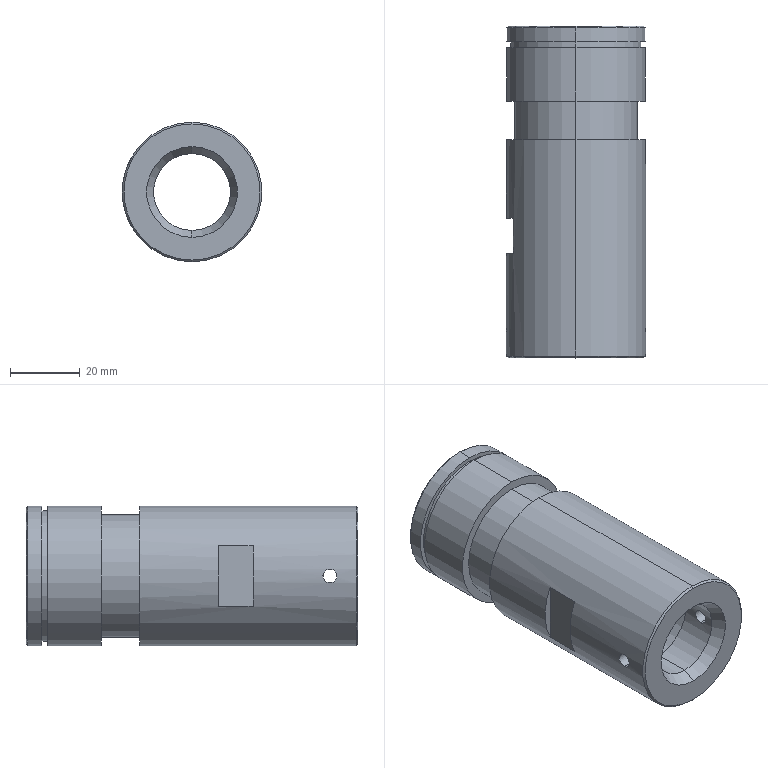Part | SolidWorks | features Chamfer 2, ICE 2, 3DProfileFeature 1, Extrusion 1, HoleWzd 1, RevCut 1 | 1 solid | 36 faces | box 40 x 95 x 40 mm | volume 59618 mm3 | cylinder 18 | plane 10 | cone 8 | commonest cylinder face diameters 40 x6 4 x4 22 x2 28 x2 35 x2 37.5 x2
STEP:
#1=CARTESIAN_POINT('',(0.,91.536,-14.));
#2=VERTEX_POINT('',#1);
#3=CARTESIAN_POINT('',(0.,91.536,14.));
#4=VERTEX_POINT('',#3);
#5=CARTESIAN_POINT('',(0.,91.536,0.));
#6=DIRECTION('',(0.,1.,0.));
#7=DIRECTION('',(0.,0.,1.));
#8=AXIS2_PLACEMENT_3D('',#5,#6,#7);
#9=CIRCLE('',#8,14.);
#10=EDGE_CURVE('',#2,#4,#9,.T.);
#11=ORIENTED_EDGE('',*,*,#10,.F.);
#12=CARTESIAN_POINT('',(0.,95.,-16.));
#13=VERTEX_POINT('',#12);
#14=CARTESIAN_POINT('',(0.,91.536,-14.));
#15=DIRECTION('',(0.,0.866,-0.5));
#16=VECTOR('',#15,1000.);
#17=LINE('',#14,#16);
#18=EDGE_CURVE('',#2,#13,#17,.T.);
#19=ORIENTED_EDGE('',*,*,#18,.T.);
#20=CARTESIAN_POINT('',(0.,95.,16.));
#21=VERTEX_POINT('',#20);
#22=CARTESIAN_POINT('',(0.,95.,0.));
#23=DIRECTION('',(0.,-1.,0.));
#24=DIRECTION('',(0.,0.,1.));
#25=AXIS2_PLACEMENT_3D('',#22,#23,#24);
#26=CIRCLE('',#25,16.);
#27=EDGE_CURVE('',#21,#13,#26,.T.);
#28=ORIENTED_EDGE('',*,*,#27,.F.);
#29=CARTESIAN_POINT('',(0.,91.536,14.));
#30=DIRECTION('',(0.,0.866,0.5));
#31=VECTOR('',#30,1000.);
#32=LINE('',#29,#31);
#33=EDGE_CURVE('',#4,#21,#32,.T.);
#34=ORIENTED_EDGE('',*,*,#33,.F.);
#35=EDGE_LOOP('',(#11,#19,#28,#34));
#36=FACE_OUTER_BOUND('',#35,.T.);
#37=CARTESIAN_POINT('',(0.,91.536,0.));
#38=DIRECTION('',(0.,1.,0.));
#39=DIRECTION('',(0.,0.,1.));
#40=AXIS2_PLACEMENT_3D('',#37,#38,#39);
#41=CONICAL_SURFACE('',#40,14.,0.5236);
#42=ADVANCED_FACE('',(#36),#41,.F.);
#43=CARTESIAN_POINT('',(0.,3.464,11.));
#44=VERTEX_POINT('',#43);
#45=CARTESIAN_POINT('',(0.,3.464,-11.));
#46=VERTEX_POINT('',#45);
#47=CARTESIAN_POINT('',(0.,3.464,0.));
#48=DIRECTION('',(0.,-1.,0.));
#49=DIRECTION('',(0.,0.,1.));
#50=AXIS2_PLACEMENT_3D('',#47,#48,#49);
#51=CIRCLE('',#50,11.);
#52=EDGE_CURVE('',#44,#46,#51,.T.);
#53=ORIENTED_EDGE('',*,*,#52,.F.);
#54=CARTESIAN_POINT('',(0.,0.,13.));
#55=VERTEX_POINT('',#54);
#56=CARTESIAN_POINT('',(0.,3.464,11.));
#57=DIRECTION('',(0.,-0.866,0.5));
#58=VECTOR('',#57,1000.);
#59=LINE('',#56,#58);
#60=EDGE_CURVE('',#44,#55,#59,.T.);
#61=ORIENTED_EDGE('',*,*,#60,.T.);
#62=CARTESIAN_POINT('',(0.,0.,-13.));
#63=VERTEX_POINT('',#62);
#64=CARTESIAN_POINT('',(0.,0.,0.));
#65=DIRECTION('',(0.,1.,0.));
#66=DIRECTION('',(0.,0.,1.));
#67=AXIS2_PLACEMENT_3D('',#64,#65,#66);
#68=CIRCLE('',#67,13.);
#69=EDGE_CURVE('',#63,#55,#68,.T.);
#70=ORIENTED_EDGE('',*,*,#69,.F.);
#71=CARTESIAN_POINT('',(0.,3.464,-11.));
#72=DIRECTION('',(0.,-0.866,-0.5));
#73=VECTOR('',#72,1000.);
#74=LINE('',#71,#73);
#75=EDGE_CURVE('',#46,#63,#74,.T.);
#76=ORIENTED_EDGE('',*,*,#75,.F.);
#77=EDGE_LOOP('',(#53,#61,#70,#76));
#78=FACE_OUTER_BOUND('',#77,.T.);
#79=CARTESIAN_POINT('',(0.,3.464,0.));
#80=DIRECTION('',(0.,-1.,0.));
#81=DIRECTION('',(0.,0.,-1.));
#82=AXIS2_PLACEMENT_3D('',#79,#80,#81);
#83=CONICAL_SURFACE('',#82,11.,0.5236);
#84=ADVANCED_FACE('',(#78),#83,.F.);
#85=CARTESIAN_POINT('',(-19.9,8.,2.));
#86=VERTEX_POINT('',#85);
#87=CARTESIAN_POINT('',(-19.9,8.,-2.));
#88=VERTEX_POINT('',#87);
#89=CARTESIAN_POINT('',(-19.9,8.,2.));
#90=CARTESIAN_POINT('',(-19.9,7.868,2.));
#91=CARTESIAN_POINT('',(-19.901,7.738,1.987));
#92=CARTESIAN_POINT('',(-19.906,7.482,1.936));
#93=CARTESIAN_POINT('',(-19.91,7.355,1.898));
#94=CARTESIAN_POINT('',(-19.919,7.113,1.797));
#95=CARTESIAN_POINT('',(-19.925,6.998,1.736));
#96=CARTESIAN_POINT('',(-19.937,6.781,1.591));
#97=CARTESIAN_POINT('',(-19.943,6.678,1.506));
#98=CARTESIAN_POINT('',(-19.963,6.401,1.23));
#99=CARTESIAN_POINT('',(-19.976,6.252,1.007));
#100=CARTESIAN_POINT('',(-19.995,6.053,0.5256));
#101=CARTESIAN_POINT('',(-20.,6.,0.2629));
#102=CARTESIAN_POINT('',(-20.,6.,-0.1337));
#103=CARTESIAN_POINT('',(-19.999,6.013,-0.2637));
#104=CARTESIAN_POINT('',(-19.994,6.064,-0.5193));
#105=CARTESIAN_POINT('',(-19.99,6.103,-0.6463));
#106=CARTESIAN_POINT('',(-19.981,6.203,-0.8884));
#107=CARTESIAN_POINT('',(-19.975,6.265,-1.003));
#108=CARTESIAN_POINT('',(-19.963,6.41,-1.22));
#109=CARTESIAN_POINT('',(-19.956,6.495,-1.323));
#110=CARTESIAN_POINT('',(-19.937,6.771,-1.599));
#111=CARTESIAN_POINT('',(-19.924,6.994,-1.748));
#112=CARTESIAN_POINT('',(-19.905,7.476,-1.948));
#113=CARTESIAN_POINT('',(-19.9,7.739,-2.));
#114=CARTESIAN_POINT('',(-19.9,8.,-2.));
#115=B_SPLINE_CURVE_WITH_KNOTS('',3,(#89,#90,#91,#92,#93,#94,#95,#96,#97,#98,#99,#100,#101,#102,#103,#104,#105,#106,#107,#108,#109,#110,#111,#112,#113,#114),.UNSPECIFIED.,.F.,.F.,(4,2,2,2,2,2,2,2,2,2,2,2,4),(0.009386,0.009777,0.01017,0.01056,0.01095,0.01173,0.01251,0.0129,0.0133,0.01369,0.01408,0.01486,0.01564),.UNSPECIFIED.);
#116=EDGE_CURVE('',#86,#88,#115,.T.);
#117=ORIENTED_EDGE('',*,*,#116,.F.);
#118=CARTESIAN_POINT('',(-10.817,8.,2.));
#119=VERTEX_POINT('',#118);
#120=CARTESIAN_POINT('',(20.,8.,2.));
#121=DIRECTION('',(1.,0.,0.));
#122=VECTOR('',#121,1000.);
#123=LINE('',#120,#122);
#124=EDGE_CURVE('',#86,#119,#123,.T.);
#125=ORIENTED_EDGE('',*,*,#124,.T.);
#126=CARTESIAN_POINT('',(-10.817,8.,-2.));
#127=VERTEX_POINT('',#126);
#128=CARTESIAN_POINT('',(-10.817,8.,-2.));
#129=CARTESIAN_POINT('',(-10.817,7.868,-2.));
#130=CARTESIAN_POINT('',(-10.819,7.737,-1.987));
#131=CARTESIAN_POINT('',(-10.828,7.481,-1.936));
#132=CARTESIAN_POINT('',(-10.835,7.354,-1.897));
#133=CARTESIAN_POINT('',(-10.852,7.112,-1.797));
#134=CARTESIAN_POINT('',(-10.862,6.997,-1.735));
#135=CARTESIAN_POINT('',(-10.885,6.78,-1.59));
#136=CARTESIAN_POINT('',(-10.897,6.678,-1.506));
#137=CARTESIAN_POINT('',(-10.933,6.401,-1.23));
#138=CARTESIAN_POINT('',(-10.956,6.253,-1.007));
#139=CARTESIAN_POINT('',(-10.99,6.053,-0.5259));
#140=CARTESIAN_POINT('',(-11.,6.,-0.2623));
#141=CARTESIAN_POINT('',(-11.,6.,0.13));
#142=CARTESIAN_POINT('',(-10.998,6.013,0.2628));
#143=CARTESIAN_POINT('',(-10.988,6.064,0.5196));
#144=CARTESIAN_POINT('',(-10.982,6.102,0.6444));
#145=CARTESIAN_POINT('',(-10.965,6.203,0.8869));
#146=CARTESIAN_POINT('',(-10.955,6.265,1.004));
#147=CARTESIAN_POINT('',(-10.933,6.41,1.22));
#148=CARTESIAN_POINT('',(-10.921,6.493,1.321));
#149=CARTESIAN_POINT('',(-10.897,6.679,1.507));
#150=CARTESIAN_POINT('',(-10.885,6.78,1.59));
#151=CARTESIAN_POINT('',(-10.863,6.996,1.735));
#152=CARTESIAN_POINT('',(-10.852,7.113,1.797));
#153=CARTESIAN_POINT('',(-10.835,7.355,1.898));
#154=CARTESIAN_POINT('',(-10.828,7.48,1.936));
#155=CARTESIAN_POINT('',(-10.819,7.737,1.987));
#156=CARTESIAN_POINT('',(-10.817,7.869,2.));
#157=CARTESIAN_POINT('',(-10.817,8.,2.));
#158=B_SPLINE_CURVE_WITH_KNOTS('',3,(#128,#129,#130,#131,#132,#133,#134,#135,#136,#137,#138,#139,#140,#141,#142,#143,#144,#145,#146,#147,#148,#149,#150,#151,#152,#153,#154,#155,#156,#157),.UNSPECIFIED.,.F.,.F.,(4,2,2,2,2,2,2,2,2,2,2,2,2,2,4),(0.,0.0003916,0.0007832,0.001175,0.001566,0.00235,0.003133,0.003525,0.003916,0.004308,0.004699,0.005091,0.005483,0.005874,0.006266),.UNSPECIFIED.);
#159=EDGE_CURVE('',#127,#119,#158,.T.);
#160=ORIENTED_EDGE('',*,*,#159,.F.);
#161=CARTESIAN_POINT('',(20.,8.,-2.));
#162=DIRECTION('',(1.,0.,0.));
#163=VECTOR('',#162,1000.);
#164=LINE('',#161,#163);
#165=EDGE_CURVE('',#88,#127,#164,.T.);
#166=ORIENTED_EDGE('',*,*,#165,.F.);
#167=EDGE_LOOP('',(#117,#125,#160,#166));
#168=FACE_OUTER_BOUND('',#167,.T.);
#169=CARTESIAN_POINT('',(20.,8.,0.));
#170=DIRECTION('',(1.,0.,0.));
#171=DIRECTION('',(0.,0.,-1.));
#172=AXIS2_PLACEMENT_3D('',#169,#170,#171);
#173=CYLINDRICAL_SURFACE('',#172,2.);
#174=ADVANCED_FACE('',(#168),#173,.F.);
#175=CARTESIAN_POINT('',(10.817,8.,2.));
#176=VERTEX_POINT('',#175);
#177=CARTESIAN_POINT('',(10.817,8.,-2.));
#178=VERTEX_POINT('',#177);
#179=CARTESIAN_POINT('',(10.817,8.,2.));
#180=CARTESIAN_POINT('',(10.817,7.739,2.));
#181=CARTESIAN_POINT('',(10.827,7.475,1.947));
#182=CARTESIAN_POINT('',(10.852,7.114,1.798));
#183=CARTESIAN_POINT('',(10.862,6.997,1.735));
#184=CARTESIAN_POINT('',(10.885,6.779,1.59));
#185=CARTESIAN_POINT('',(10.897,6.679,1.507));
#186=CARTESIAN_POINT('',(10.921,6.494,1.323));
#187=CARTESIAN_POINT('',(10.933,6.41,1.22));
#188=CARTESIAN_POINT('',(10.955,6.265,1.004));
#189=CARTESIAN_POINT('',(10.965,6.204,0.889));
#190=CARTESIAN_POINT('',(10.99,6.052,0.5252));
#191=CARTESIAN_POINT('',(11.,6.,0.2653));
#192=CARTESIAN_POINT('',(11.,6.,-0.131));
#193=CARTESIAN_POINT('',(10.998,6.013,-0.261));
#194=CARTESIAN_POINT('',(10.989,6.064,-0.5172));
#195=CARTESIAN_POINT('',(10.982,6.102,-0.6446));
#196=CARTESIAN_POINT('',(10.965,6.202,-0.8864));
#197=CARTESIAN_POINT('',(10.955,6.264,-1.001));
#198=CARTESIAN_POINT('',(10.933,6.409,-1.219));
#199=CARTESIAN_POINT('',(10.921,6.493,-1.321));
#200=CARTESIAN_POINT('',(10.885,6.769,-1.597));
#201=CARTESIAN_POINT('',(10.861,6.991,-1.747));
#202=CARTESIAN_POINT('',(10.835,7.352,-1.897));
#203=CARTESIAN_POINT('',(10.828,7.479,-1.935));
#204=CARTESIAN_POINT('',(10.819,7.737,-1.987));
#205=CARTESIAN_POINT('',(10.817,7.868,-2.));
#206=CARTESIAN_POINT('',(10.817,8.,-2.));
#207=B_SPLINE_CURVE_WITH_KNOTS('',3,(#179,#180,#181,#182,#183,#184,#185,#186,#187,#188,#189,#190,#191,#192,#193,#194,#195,#196,#197,#198,#199,#200,#201,#202,#203,#204,#205,#206),.UNSPECIFIED.,.F.,.F.,(4,2,2,2,2,2,2,2,2,2,2,2,2,4),(0.006266,0.007049,0.007441,0.007832,0.008224,0.008615,0.009398,0.00979,0.01018,0.01057,0.01096,0.01175,0.01214,0.01253),.UNSPECIFIED.);
#208=EDGE_CURVE('',#176,#178,#207,.T.);
#209=ORIENTED_EDGE('',*,*,#208,.F.);
#210=CARTESIAN_POINT('',(19.9,8.,2.));
#211=VERTEX_POINT('',#210);
#212=CARTESIAN_POINT('',(20.,8.,2.));
#213=DIRECTION('',(1.,0.,0.));
#214=VECTOR('',#213,1000.);
#215=LINE('',#212,#214);
#216=EDGE_CURVE('',#176,#211,#215,.T.);
#217=ORIENTED_EDGE('',*,*,#216,.T.);
#218=CARTESIAN_POINT('',(19.9,8.,-2.));
#219=VERTEX_POINT('',#218);
#220=CARTESIAN_POINT('',(19.9,8.,-2.));
#221=CARTESIAN_POINT('',(19.9,7.868,-2.));
#222=CARTESIAN_POINT('',(19.901,7.738,-1.987));
#223=CARTESIAN_POINT('',(19.906,7.482,-1.936));
#224=CARTESIAN_POINT('',(19.91,7.355,-1.898));
#225=CARTESIAN_POINT('',(19.919,7.113,-1.797));
#226=CARTESIAN_POINT('',(19.925,6.998,-1.736));
#227=CARTESIAN_POINT('',(19.937,6.781,-1.591));
#228=CARTESIAN_POINT('',(19.943,6.678,-1.506));
#229=CARTESIAN_POINT('',(19.963,6.401,-1.23));
#230=CARTESIAN_POINT('',(19.976,6.252,-1.006));
#231=CARTESIAN_POINT('',(19.995,6.053,-0.5251));
#232=CARTESIAN_POINT('',(20.,6.,-0.2618));
#233=CARTESIAN_POINT('',(20.,6.,0.1298));
#234=CARTESIAN_POINT('',(19.999,6.013,0.2624));
#235=CARTESIAN_POINT('',(19.994,6.064,0.519));
#236=CARTESIAN_POINT('',(19.99,6.102,0.6437));
#237=CARTESIAN_POINT('',(19.981,6.202,0.886));
#238=CARTESIAN_POINT('',(19.975,6.265,1.003));
#239=CARTESIAN_POINT('',(19.963,6.41,1.22));
#240=CARTESIAN_POINT('',(19.957,6.492,1.321));
#241=CARTESIAN_POINT('',(19.943,6.679,1.507));
#242=CARTESIAN_POINT('',(19.937,6.78,1.59));
#243=CARTESIAN_POINT('',(19.925,6.996,1.735));
#244=CARTESIAN_POINT('',(19.919,7.113,1.798));
#245=CARTESIAN_POINT('',(19.91,7.356,1.898));
#246=CARTESIAN_POINT('',(19.906,7.48,1.936));
#247=CARTESIAN_POINT('',(19.901,7.737,1.987));
#248=CARTESIAN_POINT('',(19.9,7.869,2.));
#249=CARTESIAN_POINT('',(19.9,8.,2.));
#250=B_SPLINE_CURVE_WITH_KNOTS('',3,(#220,#221,#222,#223,#224,#225,#226,#227,#228,#229,#230,#231,#232,#233,#234,#235,#236,#237,#238,#239,#240,#241,#242,#243,#244,#245,#246,#247,#248,#249),.UNSPECIFIED.,.F.,.F.,(4,2,2,2,2,2,2,2,2,2,2,2,2,2,4),(0.,0.0003911,0.0007821,0.001173,0.001564,0.002346,0.003128,0.003519,0.003911,0.004302,0.004693,0.005084,0.005475,0.005866,0.006257),.UNSPECIFIED.);
#251=EDGE_CURVE('',#219,#211,#250,.T.);
#252=ORIENTED_EDGE('',*,*,#251,.F.);
#253=CARTESIAN_POINT('',(20.,8.,-2.));
#254=DIRECTION('',(1.,0.,0.));
#255=VECTOR('',#254,1000.);
#256=LINE('',#253,#255);
#257=EDGE_CURVE('',#178,#219,#256,.T.);
#258=ORIENTED_EDGE('',*,*,#257,.F.);
#259=EDGE_LOOP('',(#209,#217,#252,#258));
#260=FACE_OUTER_BOUND('',#259,.T.);
#261=CARTESIAN_POINT('',(20.,8.,0.));
#262=DIRECTION('',(1.,0.,0.));
#263=DIRECTION('',(0.,0.,-1.));
#264=AXIS2_PLACEMENT_3D('',#261,#262,#263);
#265=CYLINDRICAL_SURFACE('',#264,2.);
#266=ADVANCED_FACE('',(#260),#265,.F.);
#267=CARTESIAN_POINT('',(0.,0.,-19.5));
#268=VERTEX_POINT('',#267);
#269=CARTESIAN_POINT('',(0.,0.,19.5));
#270=VERTEX_POINT('',#269);
#271=CARTESIAN_POINT('',(0.,0.,0.));
#272=DIRECTION('',(0.,-1.,0.));
#273=DIRECTION('',(0.,0.,1.));
#274=AXIS2_PLACEMENT_3D('',#271,#272,#273);
#275=CIRCLE('',#274,19.5);
#276=EDGE_CURVE('',#268,#270,#275,.T.);
#277=ORIENTED_EDGE('',*,*,#276,.F.);
#278=CARTESIAN_POINT('',(0.,0.5,-20.));
#279=VERTEX_POINT('',#278);
#280=CARTESIAN_POINT('',(0.,0.5,-20.));
#281=DIRECTION('',(0.,0.7071,-0.7071));
#282=VECTOR('',#281,1000.);
#283=LINE('',#280,#282);
#284=EDGE_CURVE('',#268,#279,#283,.T.);
#285=ORIENTED_EDGE('',*,*,#284,.T.);
#286=CARTESIAN_POINT('',(0.,0.5,20.));
#287=VERTEX_POINT('',#286);
#288=CARTESIAN_POINT('',(0.,0.5,0.));
#289=DIRECTION('',(0.,1.,0.));
#290=DIRECTION('',(0.,0.,1.));
#291=AXIS2_PLACEMENT_3D('',#288,#289,#290);
#292=CIRCLE('',#291,20.);
#293=EDGE_CURVE('',#287,#279,#292,.T.);
#294=ORIENTED_EDGE('',*,*,#293,.F.);
#295=CARTESIAN_POINT('',(0.,0.5,20.));
#296=DIRECTION('',(0.,0.7071,0.7071));
#297=VECTOR('',#296,1000.);
#298=LINE('',#295,#297);
#299=EDGE_CURVE('',#270,#287,#298,.T.);
#300=ORIENTED_EDGE('',*,*,#299,.F.);
#301=EDGE_LOOP('',(#277,#285,#294,#300));
#302=FACE_OUTER_BOUND('',#301,.T.);
#303=CARTESIAN_POINT('',(0.,0.5,0.));
#304=DIRECTION('',(0.,1.,0.));
#305=DIRECTION('',(0.,0.,1.));
#306=AXIS2_PLACEMENT_3D('',#303,#304,#305);
#307=CONICAL_SURFACE('',#306,20.,0.7854);
#308=ADVANCED_FACE('',(#302),#307,.T.);
#309=CARTESIAN_POINT('',(0.,95.,19.5));
#310=VERTEX_POINT('',#309);
#311=CARTESIAN_POINT('',(0.,95.,-19.5));
#312=VERTEX_POINT('',#311);
#313=CARTESIAN_POINT('',(0.,95.,0.));
#314=DIRECTION('',(0.,1.,0.));
#315=DIRECTION('',(0.,0.,1.));
#316=AXIS2_PLACEMENT_3D('',#313,#314,#315);
#317=CIRCLE('',#316,19.5);
#318=EDGE_CURVE('',#310,#312,#317,.T.);
#319=ORIENTED_EDGE('',*,*,#318,.F.);
#320=CARTESIAN_POINT('',(0.,94.5,20.));
#321=VERTEX_POINT('',#320);
#322=CARTESIAN_POINT('',(0.,95.,19.5));
#323=DIRECTION('',(0.,-0.7071,0.7071));
#324=VECTOR('',#323,1000.);
#325=LINE('',#322,#324);
#326=EDGE_CURVE('',#310,#321,#325,.T.);
#327=ORIENTED_EDGE('',*,*,#326,.T.);
#328=CARTESIAN_POINT('',(0.,94.5,-20.));
#329=VERTEX_POINT('',#328);
#330=CARTESIAN_POINT('',(0.,94.5,0.));
#331=DIRECTION('',(0.,-1.,0.));
#332=DIRECTION('',(0.,0.,1.));
#333=AXIS2_PLACEMENT_3D('',#330,#331,#332);
#334=CIRCLE('',#333,20.);
#335=EDGE_CURVE('',#329,#321,#334,.T.);
#336=ORIENTED_EDGE('',*,*,#335,.F.);
#337=CARTESIAN_POINT('',(0.,95.,-19.5));
#338=DIRECTION('',(0.,-0.7071,-0.7071));
#339=VECTOR('',#338,1000.);
#340=LINE('',#337,#339);
#341=EDGE_CURVE('',#312,#329,#340,.T.);
#342=ORIENTED_EDGE('',*,*,#341,.F.);
#343=EDGE_LOOP('',(#319,#327,#336,#342));
#344=FACE_OUTER_BOUND('',#343,.T.);
#345=CARTESIAN_POINT('',(0.,95.,0.));
#346=DIRECTION('',(0.,-1.,0.));
#347=DIRECTION('',(0.,0.,-1.));
#348=AXIS2_PLACEMENT_3D('',#345,#346,#347);
#349=CONICAL_SURFACE('',#348,19.5,0.7854);
#350=ADVANCED_FACE('',(#344),#349,.T.);
#351=ORIENTED_EDGE('',*,*,#159,.T.);
#352=CARTESIAN_POINT('',(-10.817,8.,2.));
#353=CARTESIAN_POINT('',(-10.817,8.261,2.));
#354=CARTESIAN_POINT('',(-10.827,8.525,1.947));
#355=CARTESIAN_POINT('',(-10.852,8.886,1.798));
#356=CARTESIAN_POINT('',(-10.862,9.003,1.735));
#357=CARTESIAN_POINT('',(-10.885,9.221,1.59));
#358=CARTESIAN_POINT('',(-10.897,9.321,1.507));
#359=CARTESIAN_POINT('',(-10.921,9.506,1.323));
#360=CARTESIAN_POINT('',(-10.933,9.59,1.22));
#361=CARTESIAN_POINT('',(-10.955,9.735,1.004));
#362=CARTESIAN_POINT('',(-10.965,9.796,0.889));
#363=CARTESIAN_POINT('',(-10.99,9.948,0.5252));
#364=CARTESIAN_POINT('',(-11.,10.,0.2653));
#365=CARTESIAN_POINT('',(-11.,10.,-0.131));
#366=CARTESIAN_POINT('',(-10.998,9.987,-0.261));
#367=CARTESIAN_POINT('',(-10.989,9.936,-0.5172));
#368=CARTESIAN_POINT('',(-10.982,9.898,-0.6446));
#369=CARTESIAN_POINT('',(-10.965,9.798,-0.8864));
#370=CARTESIAN_POINT('',(-10.955,9.736,-1.001));
#371=CARTESIAN_POINT('',(-10.933,9.591,-1.219));
#372=CARTESIAN_POINT('',(-10.921,9.507,-1.321));
#373=CARTESIAN_POINT('',(-10.885,9.231,-1.597));
#374=CARTESIAN_POINT('',(-10.861,9.009,-1.747));
#375=CARTESIAN_POINT('',(-10.835,8.648,-1.897));
#376=CARTESIAN_POINT('',(-10.828,8.521,-1.935));
#377=CARTESIAN_POINT('',(-10.819,8.263,-1.987));
#378=CARTESIAN_POINT('',(-10.817,8.132,-2.));
#379=CARTESIAN_POINT('',(-10.817,8.,-2.));
#380=B_SPLINE_CURVE_WITH_KNOTS('',3,(#352,#353,#354,#355,#356,#357,#358,#359,#360,#361,#362,#363,#364,#365,#366,#367,#368,#369,#370,#371,#372,#373,#374,#375,#376,#377,#378,#379),.UNSPECIFIED.,.F.,.F.,(4,2,2,2,2,2,2,2,2,2,2,2,2,4),(0.006266,0.007049,0.007441,0.007832,0.008224,0.008615,0.009398,0.00979,0.01018,0.01057,0.01096,0.01175,0.01214,0.01253),.UNSPECIFIED.);
#381=EDGE_CURVE('',#119,#127,#380,.T.);
#382=ORIENTED_EDGE('',*,*,#381,.T.);
#383=EDGE_LOOP('',(#351,#382));
#384=FACE_BOUND('',#383,.T.);
#385=CARTESIAN_POINT('',(0.,14.,11.));
#386=VERTEX_POINT('',#385);
#387=CARTESIAN_POINT('',(0.,14.,-11.));
#388=VERTEX_POINT('',#387);
#389=CARTESIAN_POINT('',(0.,14.,0.));
#390=DIRECTION('',(0.,-1.,0.));
#391=DIRECTION('',(0.,0.,-1.));
#392=AXIS2_PLACEMENT_3D('',#389,#390,#391);
#393=CIRCLE('',#392,11.);
#394=EDGE_CURVE('',#386,#388,#393,.T.);
#395=ORIENTED_EDGE('',*,*,#394,.F.);
#396=CARTESIAN_POINT('',(0.,14.,11.));
#397=DIRECTION('',(0.,-1.,0.));
#398=VECTOR('',#397,1000.);
#399=LINE('',#396,#398);
#400=EDGE_CURVE('',#386,#44,#399,.T.);
#401=ORIENTED_EDGE('',*,*,#400,.T.);
#402=ORIENTED_EDGE('',*,*,#52,.T.);
#403=CARTESIAN_POINT('',(0.,14.,-11.));
#404=DIRECTION('',(0.,-1.,0.));
#405=VECTOR('',#404,1000.);
#406=LINE('',#403,#405);
#407=EDGE_CURVE('',#388,#46,#406,.T.);
#408=ORIENTED_EDGE('',*,*,#407,.F.);
#409=EDGE_LOOP('',(#395,#401,#402,#408));
#410=FACE_OUTER_BOUND('',#409,.T.);
#411=CARTESIAN_POINT('',(0.,14.,0.));
#412=DIRECTION('',(0.,-1.,0.));
#413=DIRECTION('',(0.,0.,-1.));
#414=AXIS2_PLACEMENT_3D('',#411,#412,#413);
#415=CYLINDRICAL_SURFACE('',#414,11.);
#416=ADVANCED_FACE('',(#384,#410),#415,.F.);
#417=CARTESIAN_POINT('',(0.,90.5,-18.75));
#418=VERTEX_POINT('',#417);
#419=CARTESIAN_POINT('',(0.,90.5,18.75));
#420=VERTEX_POINT('',#419);
#421=CARTESIAN_POINT('',(0.,90.5,0.));
#422=DIRECTION('',(0.,-1.,0.));
#423=DIRECTION('',(0.,0.,-1.));
#424=AXIS2_PLACEMENT_3D('',#421,#422,#423);
#425=CIRCLE('',#424,18.75);
#426=EDGE_CURVE('',#418,#420,#425,.T.);
#427=ORIENTED_EDGE('',*,*,#426,.T.);
#428=CARTESIAN_POINT('',(0.,88.8,18.75));
#429=VERTEX_POINT('',#428);
#430=CARTESIAN_POINT('',(0.,0.,18.75));
#431=DIRECTION('',(0.,-1.,0.));
#432=VECTOR('',#431,1000.);
#433=LINE('',#430,#432);
#434=EDGE_CURVE('',#420,#429,#433,.T.);
#435=ORIENTED_EDGE('',*,*,#434,.T.);
#436=CARTESIAN_POINT('',(0.,88.8,-18.75));
#437=VERTEX_POINT('',#436);
#438=CARTESIAN_POINT('',(0.,88.8,0.));
#439=DIRECTION('',(0.,-1.,0.));
#440=DIRECTION('',(0.,0.,-1.));
#441=AXIS2_PLACEMENT_3D('',#438,#439,#440);
#442=CIRCLE('',#441,18.75);
#443=EDGE_CURVE('',#437,#429,#442,.T.);
#444=ORIENTED_EDGE('',*,*,#443,.F.);
#445=CARTESIAN_POINT('',(0.,0.,-18.75));
#446=DIRECTION('',(0.,-1.,0.));
#447=VECTOR('',#446,1000.);
#448=LINE('',#445,#447);
#449=EDGE_CURVE('',#418,#437,#448,.T.);
#450=ORIENTED_EDGE('',*,*,#449,.F.);
#451=EDGE_LOOP('',(#427,#435,#444,#450));
#452=FACE_OUTER_BOUND('',#451,.T.);
#453=CARTESIAN_POINT('',(0.,0.,0.));
#454=DIRECTION('',(0.,-1.,0.));
#455=DIRECTION('',(0.,0.,-1.));
#456=AXIS2_PLACEMENT_3D('',#453,#454,#455);
#457=CYLINDRICAL_SURFACE('',#456,18.75);
#458=ADVANCED_FACE('',(#452),#457,.T.);
#459=CARTESIAN_POINT('',(0.,73.5,-17.5));
#460=VERTEX_POINT('',#459);
#461=CARTESIAN_POINT('',(0.,73.5,17.5));
#462=VERTEX_POINT('',#461);
#463=CARTESIAN_POINT('',(0.,73.5,0.));
#464=DIRECTION('',(0.,-1.,0.));
#465=DIRECTION('',(0.,0.,-1.));
#466=AXIS2_PLACEMENT_3D('',#463,#464,#465);
#467=CIRCLE('',#466,17.5);
#468=EDGE_CURVE('',#460,#462,#467,.T.);
#469=ORIENTED_EDGE('',*,*,#468,.T.);
#470=CARTESIAN_POINT('',(0.,62.5,17.5));
#471=VERTEX_POINT('',#470);
#472=CARTESIAN_POINT('',(0.,0.,17.5));
#473=DIRECTION('',(0.,-1.,0.));
#474=VECTOR('',#473,1000.);
#475=LINE('',#472,#474);
#476=EDGE_CURVE('',#462,#471,#475,.T.);
#477=ORIENTED_EDGE('',*,*,#476,.T.);
#478=CARTESIAN_POINT('',(0.,62.5,-17.5));
#479=VERTEX_POINT('',#478);
#480=CARTESIAN_POINT('',(0.,62.5,0.));
#481=DIRECTION('',(0.,-1.,0.));
#482=DIRECTION('',(0.,0.,-1.));
#483=AXIS2_PLACEMENT_3D('',#480,#481,#482);
#484=CIRCLE('',#483,17.5);
#485=EDGE_CURVE('',#479,#471,#484,.T.);
#486=ORIENTED_EDGE('',*,*,#485,.F.);
#487=CARTESIAN_POINT('',(0.,0.,-17.5));
#488=DIRECTION('',(0.,-1.,0.));
#489=VECTOR('',#488,1000.);
#490=LINE('',#487,#489);
#491=EDGE_CURVE('',#460,#479,#490,.T.);
#492=ORIENTED_EDGE('',*,*,#491,.F.);
#493=EDGE_LOOP('',(#469,#477,#486,#492));
#494=FACE_OUTER_BOUND('',#493,.T.);
#495=CARTESIAN_POINT('',(0.,0.,0.));
#496=DIRECTION('',(0.,-1.,0.));
#497=DIRECTION('',(0.,0.,-1.));
#498=AXIS2_PLACEMENT_3D('',#495,#496,#497);
#499=CYLINDRICAL_SURFACE('',#498,17.5);
#500=ADVANCED_FACE('',(#494),#499,.T.);
#501=ORIENTED_EDGE('',*,*,#335,.T.);
#502=CARTESIAN_POINT('',(0.,90.5,20.));
#503=VERTEX_POINT('',#502);
#504=CARTESIAN_POINT('',(0.,95.,20.));
#505=DIRECTION('',(0.,-1.,0.));
#506=VECTOR('',#505,1000.);
#507=LINE('',#504,#506);
#508=EDGE_CURVE('',#321,#503,#507,.T.);
#509=ORIENTED_EDGE('',*,*,#508,.T.);
#510=CARTESIAN_POINT('',(0.,90.5,-20.));
#511=VERTEX_POINT('',#510);
#512=CARTESIAN_POINT('',(0.,90.5,0.));
#513=DIRECTION('',(0.,-1.,0.));
#514=DIRECTION('',(0.,0.,-1.));
#515=AXIS2_PLACEMENT_3D('',#512,#513,#514);
#516=CIRCLE('',#515,20.);
#517=EDGE_CURVE('',#511,#503,#516,.T.);
#518=ORIENTED_EDGE('',*,*,#517,.F.);
#519=CARTESIAN_POINT('',(0.,95.,-20.));
#520=DIRECTION('',(0.,-1.,0.));
#521=VECTOR('',#520,1000.);
#522=LINE('',#519,#521);
#523=EDGE_CURVE('',#329,#511,#522,.T.);
#524=ORIENTED_EDGE('',*,*,#523,.F.);
#525=EDGE_LOOP('',(#501,#509,#518,#524));
#526=FACE_OUTER_BOUND('',#525,.T.);
#527=CARTESIAN_POINT('',(0.,95.,0.));
#528=DIRECTION('',(0.,-1.,0.));
#529=DIRECTION('',(0.,0.,-1.));
#530=AXIS2_PLACEMENT_3D('',#527,#528,#529);
#531=CYLINDRICAL_SURFACE('',#530,20.);
#532=ADVANCED_FACE('',(#526),#531,.T.);
#533=ORIENTED_EDGE('',*,*,#251,.T.);
#534=CARTESIAN_POINT('',(19.9,8.,2.));
#535=CARTESIAN_POINT('',(19.9,8.261,2.));
#536=CARTESIAN_POINT('',(19.905,8.524,1.948));
#537=CARTESIAN_POINT('',(19.924,9.006,1.748));
#538=CARTESIAN_POINT('',(19.937,9.229,1.599));
#539=CARTESIAN_POINT('',(19.956,9.505,1.323));
#540=CARTESIAN_POINT('',(19.963,9.59,1.22));
#541=CARTESIAN_POINT('',(19.975,9.735,1.003));
#542=CARTESIAN_POINT('',(19.981,9.797,0.8883));
#543=CARTESIAN_POINT('',(19.99,9.897,0.6463));
#544=CARTESIAN_POINT('',(19.994,9.936,0.5192));
#545=CARTESIAN_POINT('',(19.999,9.987,0.2636));
#546=CARTESIAN_POINT('',(20.,10.,0.1337));
#547=CARTESIAN_POINT('',(20.,10.,-0.1306));
#548=CARTESIAN_POINT('',(19.999,9.987,-0.2608));
#549=CARTESIAN_POINT('',(19.994,9.937,-0.5165));
#550=CARTESIAN_POINT('',(19.99,9.898,-0.6435));
#551=CARTESIAN_POINT('',(19.981,9.798,-0.8858));
#552=CARTESIAN_POINT('',(19.975,9.737,-1.001));
#553=CARTESIAN_POINT('',(19.963,9.592,-1.218));
#554=CARTESIAN_POINT('',(19.957,9.507,-1.321));
#555=CARTESIAN_POINT('',(19.937,9.231,-1.598));
#556=CARTESIAN_POINT('',(19.924,9.008,-1.747));
#557=CARTESIAN_POINT('',(19.905,8.527,-1.947));
#558=CARTESIAN_POINT('',(19.9,8.264,-2.));
#559=CARTESIAN_POINT('',(19.9,8.,-2.));
#560=B_SPLINE_CURVE_WITH_KNOTS('',3,(#534,#535,#536,#537,#538,#539,#540,#541,#542,#543,#544,#545,#546,#547,#548,#549,#550,#551,#552,#553,#554,#555,#556,#557,#558,#559),.UNSPECIFIED.,.F.,.F.,(4,2,2,2,2,2,2,2,2,2,2,2,4),(0.006257,0.007039,0.007821,0.008212,0.008603,0.008994,0.009384,0.009775,0.01017,0.01056,0.01095,0.01173,0.01251),.UNSPECIFIED.);
#561=EDGE_CURVE('',#211,#219,#560,.T.);
#562=ORIENTED_EDGE('',*,*,#561,.T.);
#563=EDGE_LOOP('',(#533,#562));
#564=FACE_BOUND('',#563,.T.);
#565=CARTESIAN_POINT('',(0.,62.5,-20.));
#566=VERTEX_POINT('',#565);
#567=CARTESIAN_POINT('',(0.,62.5,20.));
#568=VERTEX_POINT('',#567);
#569=CARTESIAN_POINT('',(0.,62.5,0.));
#570=DIRECTION('',(0.,-1.,0.));
#571=DIRECTION('',(0.,0.,-1.));
#572=AXIS2_PLACEMENT_3D('',#569,#570,#571);
#573=CIRCLE('',#572,20.);
#574=EDGE_CURVE('',#566,#568,#573,.T.);
#575=ORIENTED_EDGE('',*,*,#574,.T.);
#576=CARTESIAN_POINT('',(0.,95.,20.));
#577=DIRECTION('',(0.,-1.,0.));
#578=VECTOR('',#577,1000.);
#579=LINE('',#576,#578);
#580=EDGE_CURVE('',#568,#287,#579,.T.);
#581=ORIENTED_EDGE('',*,*,#580,.T.);
#582=ORIENTED_EDGE('',*,*,#293,.T.);
#583=CARTESIAN_POINT('',(0.,95.,-20.));
#584=DIRECTION('',(0.,-1.,0.));
#585=VECTOR('',#584,1000.);
#586=LINE('',#583,#585);
#587=EDGE_CURVE('',#566,#279,#586,.T.);
#588=ORIENTED_EDGE('',*,*,#587,.F.);
#589=EDGE_LOOP('',(#575,#581,#582,#588));
#590=FACE_OUTER_BOUND('',#589,.T.);
#591=CARTESIAN_POINT('',(0.,95.,0.));
#592=DIRECTION('',(0.,-1.,0.));
#593=DIRECTION('',(0.,0.,-1.));
#594=AXIS2_PLACEMENT_3D('',#591,#592,#593);
#595=CYLINDRICAL_SURFACE('',#594,20.);
#596=ADVANCED_FACE('',(#564,#590),#595,.T.);
#597=CARTESIAN_POINT('',(0.,88.8,-20.));
#598=VERTEX_POINT('',#597);
#599=CARTESIAN_POINT('',(0.,88.8,20.));
#600=VERTEX_POINT('',#599);
#601=CARTESIAN_POINT('',(0.,88.8,0.));
#602=DIRECTION('',(0.,-1.,0.));
#603=DIRECTION('',(0.,0.,-1.));
#604=AXIS2_PLACEMENT_3D('',#601,#602,#603);
#605=CIRCLE('',#604,20.);
#606=EDGE_CURVE('',#598,#600,#605,.T.);
#607=ORIENTED_EDGE('',*,*,#606,.T.);
#608=CARTESIAN_POINT('',(0.,73.5,20.));
#609=VERTEX_POINT('',#608);
#610=CARTESIAN_POINT('',(0.,95.,20.));
#611=DIRECTION('',(0.,-1.,0.));
#612=VECTOR('',#611,1000.);
#613=LINE('',#610,#612);
#614=EDGE_CURVE('',#600,#609,#613,.T.);
#615=ORIENTED_EDGE('',*,*,#614,.T.);
#616=CARTESIAN_POINT('',(0.,73.5,-20.));
#617=VERTEX_POINT('',#616);
#618=CARTESIAN_POINT('',(0.,73.5,0.));
#619=DIRECTION('',(0.,-1.,0.));
#620=DIRECTION('',(0.,0.,-1.));
#621=AXIS2_PLACEMENT_3D('',#618,#619,#620);
#622=CIRCLE('',#621,20.);
#623=EDGE_CURVE('',#617,#609,#622,.T.);
#624=ORIENTED_EDGE('',*,*,#623,.F.);
#625=CARTESIAN_POINT('',(0.,95.,-20.));
#626=DIRECTION('',(0.,-1.,0.));
#627=VECTOR('',#626,1000.);
#628=LINE('',#625,#627);
#629=EDGE_CURVE('',#598,#617,#628,.T.);
#630=ORIENTED_EDGE('',*,*,#629,.F.);
#631=EDGE_LOOP('',(#607,#615,#624,#630));
#632=FACE_OUTER_BOUND('',#631,.T.);
#633=CARTESIAN_POINT('',(0.,95.,0.));
#634=DIRECTION('',(0.,-1.,0.));
#635=DIRECTION('',(0.,0.,-1.));
#636=AXIS2_PLACEMENT_3D('',#633,#634,#635);
#637=CYLINDRICAL_SURFACE('',#636,20.);
#638=ADVANCED_FACE('',(#632),#637,.T.);
#639=ORIENTED_EDGE('',*,*,#10,.T.);
#640=CARTESIAN_POINT('',(0.,14.,14.));
#641=VERTEX_POINT('',#640);
#642=CARTESIAN_POINT('',(0.,95.,14.));
#643=DIRECTION('',(0.,-1.,0.));
#644=VECTOR('',#643,1000.);
#645=LINE('',#642,#644);
#646=EDGE_CURVE('',#4,#641,#645,.T.);
#647=ORIENTED_EDGE('',*,*,#646,.T.);
#648=CARTESIAN_POINT('',(0.,14.,-14.));
#649=VERTEX_POINT('',#648);
#650=CARTESIAN_POINT('',(0.,14.,0.));
#651=DIRECTION('',(0.,-1.,0.));
#652=DIRECTION('',(0.,0.,-1.));
#653=AXIS2_PLACEMENT_3D('',#650,#651,#652);
#654=CIRCLE('',#653,14.);
#655=EDGE_CURVE('',#641,#649,#654,.T.);
#656=ORIENTED_EDGE('',*,*,#655,.T.);
#657=CARTESIAN_POINT('',(0.,95.,-14.));
#658=DIRECTION('',(0.,-1.,0.));
#659=VECTOR('',#658,1000.);
#660=LINE('',#657,#659);
#661=EDGE_CURVE('',#2,#649,#660,.T.);
#662=ORIENTED_EDGE('',*,*,#661,.F.);
#663=EDGE_LOOP('',(#639,#647,#656,#662));
#664=FACE_OUTER_BOUND('',#663,.T.);
#665=CARTESIAN_POINT('',(0.,95.,0.));
#666=DIRECTION('',(0.,-1.,0.));
#667=DIRECTION('',(0.,0.,-1.));
#668=AXIS2_PLACEMENT_3D('',#665,#666,#667);
#669=CYLINDRICAL_SURFACE('',#668,14.);
#670=ADVANCED_FACE('',(#664),#669,.F.);
#671=ORIENTED_EDGE('',*,*,#646,.F.);
#672=CARTESIAN_POINT('',(0.,91.536,0.));
#673=DIRECTION('',(0.,1.,0.));
#674=DIRECTION('',(0.,0.,1.));
#675=AXIS2_PLACEMENT_3D('',#672,#673,#674);
#676=CIRCLE('',#675,14.);
#677=EDGE_CURVE('',#4,#2,#676,.T.);
#678=ORIENTED_EDGE('',*,*,#677,.T.);
#679=ORIENTED_EDGE('',*,*,#661,.T.);
#680=CARTESIAN_POINT('',(0.,14.,0.));
#681=DIRECTION('',(0.,-1.,0.));
#682=DIRECTION('',(0.,0.,-1.));
#683=AXIS2_PLACEMENT_3D('',#680,#681,#682);
#684=CIRCLE('',#683,14.);
#685=EDGE_CURVE('',#649,#641,#684,.T.);
#686=ORIENTED_EDGE('',*,*,#685,.T.);
#687=EDGE_LOOP('',(#671,#678,#679,#686));
#688=FACE_OUTER_BOUND('',#687,.T.);
#689=CARTESIAN_POINT('',(0.,95.,0.));
#690=DIRECTION('',(0.,-1.,0.));
#691=DIRECTION('',(0.,0.,-1.));
#692=AXIS2_PLACEMENT_3D('',#689,#690,#691);
#693=CYLINDRICAL_SURFACE('',#692,14.);
#694=ADVANCED_FACE('',(#688),#693,.F.);
#695=ORIENTED_EDGE('',*,*,#614,.F.);
#696=CARTESIAN_POINT('',(0.,88.8,0.));
#697=DIRECTION('',(0.,-1.,0.));
#698=DIRECTION('',(0.,0.,-1.));
#699=AXIS2_PLACEMENT_3D('',#696,#697,#698);
#700=CIRCLE('',#699,20.);
#701=EDGE_CURVE('',#600,#598,#700,.T.);
#702=ORIENTED_EDGE('',*,*,#701,.T.);
#703=ORIENTED_EDGE('',*,*,#629,.T.);
#704=CARTESIAN_POINT('',(0.,73.5,0.));
#705=DIRECTION('',(0.,-1.,0.));
#706=DIRECTION('',(0.,0.,-1.));
#707=AXIS2_PLACEMENT_3D('',#704,#705,#706);
#708=CIRCLE('',#707,20.);
#709=EDGE_CURVE('',#609,#617,#708,.T.);
#710=ORIENTED_EDGE('',*,*,#709,.F.);
#711=EDGE_LOOP('',(#695,#702,#703,#710));
#712=FACE_OUTER_BOUND('',#711,.T.);
#713=CARTESIAN_POINT('',(0.,95.,0.));
#714=DIRECTION('',(0.,-1.,0.));
#715=DIRECTION('',(0.,0.,-1.));
#716=AXIS2_PLACEMENT_3D('',#713,#714,#715);
#717=CYLINDRICAL_SURFACE('',#716,20.);
#718=ADVANCED_FACE('',(#712),#717,.T.);
#719=ORIENTED_EDGE('',*,*,#580,.F.);
#720=CARTESIAN_POINT('',(0.,62.5,0.));
#721=DIRECTION('',(0.,-1.,0.));
#722=DIRECTION('',(0.,0.,-1.));
#723=AXIS2_PLACEMENT_3D('',#720,#721,#722);
#724=CIRCLE('',#723,20.);
#725=EDGE_CURVE('',#568,#566,#724,.T.);
#726=ORIENTED_EDGE('',*,*,#725,.T.);
#727=ORIENTED_EDGE('',*,*,#587,.T.);
#728=CARTESIAN_POINT('',(0.,0.5,0.));
#729=DIRECTION('',(0.,1.,0.));
#730=DIRECTION('',(0.,0.,1.));
#731=AXIS2_PLACEMENT_3D('',#728,#729,#730);
#732=CIRCLE('',#731,20.);
#733=EDGE_CURVE('',#279,#287,#732,.T.);
#734=ORIENTED_EDGE('',*,*,#733,.T.);
#735=EDGE_LOOP('',(#719,#726,#727,#734));
#736=FACE_OUTER_BOUND('',#735,.T.);
#737=CARTESIAN_POINT('',(-18.,30.,-8.718));
#738=VERTEX_POINT('',#737);
#739=CARTESIAN_POINT('',(-18.,40.,-8.718));
#740=VERTEX_POINT('',#739);
#741=CARTESIAN_POINT('',(-18.,95.,-8.718));
#742=DIRECTION('',(0.,1.,0.));
#743=VECTOR('',#742,1000.);
#744=LINE('',#741,#743);
#745=EDGE_CURVE('',#738,#740,#744,.T.);
#746=ORIENTED_EDGE('',*,*,#745,.T.);
#747=CARTESIAN_POINT('',(-18.,40.,8.718));
#748=VERTEX_POINT('',#747);
#749=CARTESIAN_POINT('',(0.,40.,0.));
#750=DIRECTION('',(0.,1.,0.));
#751=DIRECTION('',(0.,0.,1.));
#752=AXIS2_PLACEMENT_3D('',#749,#750,#751);
#753=CIRCLE('',#752,20.);
#754=EDGE_CURVE('',#740,#748,#753,.T.);
#755=ORIENTED_EDGE('',*,*,#754,.T.);
#756=CARTESIAN_POINT('',(-18.,30.,8.718));
#757=VERTEX_POINT('',#756);
#758=CARTESIAN_POINT('',(-18.,95.,8.718));
#759=DIRECTION('',(0.,-1.,0.));
#760=VECTOR('',#759,1000.);
#761=LINE('',#758,#760);
#762=EDGE_CURVE('',#748,#757,#761,.T.);
#763=ORIENTED_EDGE('',*,*,#762,.T.);
#764=CARTESIAN_POINT('',(0.,30.,0.));
#765=DIRECTION('',(0.,-1.,0.));
#766=DIRECTION('',(0.,0.,-1.));
#767=AXIS2_PLACEMENT_3D('',#764,#765,#766);
#768=CIRCLE('',#767,20.);
#769=EDGE_CURVE('',#757,#738,#768,.T.);
#770=ORIENTED_EDGE('',*,*,#769,.T.);
#771=EDGE_LOOP('',(#746,#755,#763,#770));
#772=FACE_BOUND('',#771,.T.);
#773=CARTESIAN_POINT('',(-19.9,8.,-2.));
#774=CARTESIAN_POINT('',(-19.9,8.131,-2.));
#775=CARTESIAN_POINT('',(-19.901,8.263,-1.987));
#776=CARTESIAN_POINT('',(-19.906,8.52,-1.936));
#777=CARTESIAN_POINT('',(-19.91,8.644,-1.898));
#778=CARTESIAN_POINT('',(-19.919,8.887,-1.798));
#779=CARTESIAN_POINT('',(-19.925,9.004,-1.735));
#780=CARTESIAN_POINT('',(-19.937,9.22,-1.59));
#781=CARTESIAN_POINT('',(-19.943,9.321,-1.507));
#782=CARTESIAN_POINT('',(-19.957,9.508,-1.321));
#783=CARTESIAN_POINT('',(-19.963,9.591,-1.22));
#784=CARTESIAN_POINT('',(-19.975,9.735,-1.003));
#785=CARTESIAN_POINT('',(-19.981,9.798,-0.8859));
#786=CARTESIAN_POINT('',(-19.99,9.898,-0.6436));
#787=CARTESIAN_POINT('',(-19.994,9.936,-0.5189));
#788=CARTESIAN_POINT('',(-19.999,9.987,-0.2624));
#789=CARTESIAN_POINT('',(-20.,10.,-0.1298));
#790=CARTESIAN_POINT('',(-20.,10.,0.2619));
#791=CARTESIAN_POINT('',(-19.995,9.947,0.5252));
#792=CARTESIAN_POINT('',(-19.976,9.748,1.007));
#793=CARTESIAN_POINT('',(-19.963,9.599,1.23));
#794=CARTESIAN_POINT('',(-19.943,9.322,1.506));
#795=CARTESIAN_POINT('',(-19.937,9.219,1.591));
#796=CARTESIAN_POINT('',(-19.925,9.002,1.736));
#797=CARTESIAN_POINT('',(-19.919,8.887,1.797));
#798=CARTESIAN_POINT('',(-19.91,8.645,1.898));
#799=CARTESIAN_POINT('',(-19.906,8.518,1.936));
#800=CARTESIAN_POINT('',(-19.901,8.262,1.987));
#801=CARTESIAN_POINT('',(-19.9,8.132,2.));
#802=CARTESIAN_POINT('',(-19.9,8.,2.));
#803=B_SPLINE_CURVE_WITH_KNOTS('',3,(#773,#774,#775,#776,#777,#778,#779,#780,#781,#782,#783,#784,#785,#786,#787,#788,#789,#790,#791,#792,#793,#794,#795,#796,#797,#798,#799,#800,#801,#802),.UNSPECIFIED.,.F.,.F.,(4,2,2,2,2,2,2,2,2,2,2,2,2,2,4),(0.003129,0.00352,0.003911,0.004302,0.004693,0.005084,0.005475,0.005867,0.006258,0.00704,0.007822,0.008213,0.008604,0.008995,0.009386),.UNSPECIFIED.);
#804=EDGE_CURVE('',#88,#86,#803,.T.);
#805=ORIENTED_EDGE('',*,*,#804,.T.);
#806=ORIENTED_EDGE('',*,*,#116,.T.);
#807=EDGE_LOOP('',(#805,#806));
#808=FACE_BOUND('',#807,.T.);
#809=CARTESIAN_POINT('',(0.,95.,0.));
#810=DIRECTION('',(0.,-1.,0.));
#811=DIRECTION('',(0.,0.,-1.));
#812=AXIS2_PLACEMENT_3D('',#809,#810,#811);
#813=CYLINDRICAL_SURFACE('',#812,20.);
#814=ADVANCED_FACE('',(#736,#772,#808),#813,.T.);
#815=ORIENTED_EDGE('',*,*,#27,.T.);
#816=CARTESIAN_POINT('',(0.,95.,0.));
#817=DIRECTION('',(0.,-1.,0.));
#818=DIRECTION('',(0.,0.,1.));
#819=AXIS2_PLACEMENT_3D('',#816,#817,#818);
#820=CIRCLE('',#819,16.);
#821=EDGE_CURVE('',#13,#21,#820,.T.);
#822=ORIENTED_EDGE('',*,*,#821,.T.);
#823=EDGE_LOOP('',(#815,#822));
#824=FACE_BOUND('',#823,.T.);
#825=CARTESIAN_POINT('',(0.,95.,0.));
#826=DIRECTION('',(0.,1.,0.));
#827=DIRECTION('',(0.,0.,1.));
#828=AXIS2_PLACEMENT_3D('',#825,#826,#827);
#829=CIRCLE('',#828,19.5);
#830=EDGE_CURVE('',#312,#310,#829,.T.);
#831=ORIENTED_EDGE('',*,*,#830,.T.);
#832=ORIENTED_EDGE('',*,*,#318,.T.);
#833=EDGE_LOOP('',(#831,#832));
#834=FACE_OUTER_BOUND('',#833,.T.);
#835=CARTESIAN_POINT('',(0.,95.,0.));
#836=DIRECTION('',(0.,1.,0.));
#837=DIRECTION('',(0.,0.,1.));
#838=AXIS2_PLACEMENT_3D('',#835,#836,#837);
#839=PLANE('',#838);
#840=ADVANCED_FACE('',(#824,#834),#839,.T.);
#841=ORIENTED_EDGE('',*,*,#69,.T.);
#842=CARTESIAN_POINT('',(0.,0.,0.));
#843=DIRECTION('',(0.,1.,0.));
#844=DIRECTION('',(0.,0.,1.));
#845=AXIS2_PLACEMENT_3D('',#842,#843,#844);
#846=CIRCLE('',#845,13.);
#847=EDGE_CURVE('',#55,#63,#846,.T.);
#848=ORIENTED_EDGE('',*,*,#847,.T.);
#849=EDGE_LOOP('',(#841,#848));
#850=FACE_BOUND('',#849,.T.);
#851=CARTESIAN_POINT('',(0.,0.,0.));
#852=DIRECTION('',(0.,-1.,0.));
#853=DIRECTION('',(0.,0.,1.));
#854=AXIS2_PLACEMENT_3D('',#851,#852,#853);
#855=CIRCLE('',#854,19.5);
#856=EDGE_CURVE('',#270,#268,#855,.T.);
#857=ORIENTED_EDGE('',*,*,#856,.T.);
#858=ORIENTED_EDGE('',*,*,#276,.T.);
#859=EDGE_LOOP('',(#857,#858));
#860=FACE_OUTER_BOUND('',#859,.T.);
#861=CARTESIAN_POINT('',(0.,0.,0.));
#862=DIRECTION('',(0.,1.,0.));
#863=DIRECTION('',(0.,0.,1.));
#864=AXIS2_PLACEMENT_3D('',#861,#862,#863);
#865=PLANE('',#864);
#866=ADVANCED_FACE('',(#850,#860),#865,.F.);
#867=ORIENTED_EDGE('',*,*,#508,.F.);
#868=CARTESIAN_POINT('',(0.,94.5,0.));
#869=DIRECTION('',(0.,-1.,0.));
#870=DIRECTION('',(0.,0.,1.));
#871=AXIS2_PLACEMENT_3D('',#868,#869,#870);
#872=CIRCLE('',#871,20.);
#873=EDGE_CURVE('',#321,#329,#872,.T.);
#874=ORIENTED_EDGE('',*,*,#873,.T.);
#875=ORIENTED_EDGE('',*,*,#523,.T.);
#876=CARTESIAN_POINT('',(0.,90.5,0.));
#877=DIRECTION('',(0.,-1.,0.));
#878=DIRECTION('',(0.,0.,-1.));
#879=AXIS2_PLACEMENT_3D('',#876,#877,#878);
#880=CIRCLE('',#879,20.);
#881=EDGE_CURVE('',#503,#511,#880,.T.);
#882=ORIENTED_EDGE('',*,*,#881,.F.);
#883=EDGE_LOOP('',(#867,#874,#875,#882));
#884=FACE_OUTER_BOUND('',#883,.T.);
#885=CARTESIAN_POINT('',(0.,95.,0.));
#886=DIRECTION('',(0.,-1.,0.));
#887=DIRECTION('',(0.,0.,-1.));
#888=AXIS2_PLACEMENT_3D('',#885,#886,#887);
#889=CYLINDRICAL_SURFACE('',#888,20.);
#890=ADVANCED_FACE('',(#884),#889,.T.);
#891=ORIENTED_EDGE('',*,*,#574,.F.);
#892=ORIENTED_EDGE('',*,*,#725,.F.);
#893=EDGE_LOOP('',(#891,#892));
#894=FACE_OUTER_BOUND('',#893,.T.);
#895=ORIENTED_EDGE('',*,*,#485,.T.);
#896=CARTESIAN_POINT('',(0.,62.5,0.));
#897=DIRECTION('',(0.,-1.,0.));
#898=DIRECTION('',(0.,0.,-1.));
#899=AXIS2_PLACEMENT_3D('',#896,#897,#898);
#900=CIRCLE('',#899,17.5);
#901=EDGE_CURVE('',#471,#479,#900,.T.);
#902=ORIENTED_EDGE('',*,*,#901,.T.);
#903=EDGE_LOOP('',(#895,#902));
#904=FACE_BOUND('',#903,.T.);
#905=CARTESIAN_POINT('',(20.,62.5,0.));
#906=DIRECTION('',(0.,-1.,0.));
#907=DIRECTION('',(0.,0.,-1.));
#908=AXIS2_PLACEMENT_3D('',#905,#906,#907);
#909=PLANE('',#908);
#910=ADVANCED_FACE('',(#894,#904),#909,.F.);
#911=ORIENTED_EDGE('',*,*,#476,.F.);
#912=CARTESIAN_POINT('',(0.,73.5,0.));
#913=DIRECTION('',(0.,-1.,0.));
#914=DIRECTION('',(0.,0.,-1.));
#915=AXIS2_PLACEMENT_3D('',#912,#913,#914);
#916=CIRCLE('',#915,17.5);
#917=EDGE_CURVE('',#462,#460,#916,.T.);
#918=ORIENTED_EDGE('',*,*,#917,.T.);
#919=ORIENTED_EDGE('',*,*,#491,.T.);
#920=ORIENTED_EDGE('',*,*,#901,.F.);
#921=EDGE_LOOP('',(#911,#918,#919,#920));
#922=FACE_OUTER_BOUND('',#921,.T.);
#923=CARTESIAN_POINT('',(0.,0.,0.));
#924=DIRECTION('',(0.,-1.,0.));
#925=DIRECTION('',(0.,0.,-1.));
#926=AXIS2_PLACEMENT_3D('',#923,#924,#925);
#927=CYLINDRICAL_SURFACE('',#926,17.5);
#928=ADVANCED_FACE('',(#922),#927,.T.);
#929=ORIENTED_EDGE('',*,*,#468,.F.);
#930=ORIENTED_EDGE('',*,*,#917,.F.);
#931=EDGE_LOOP('',(#929,#930));
#932=FACE_BOUND('',#931,.T.);
#933=ORIENTED_EDGE('',*,*,#623,.T.);
#934=ORIENTED_EDGE('',*,*,#709,.T.);
#935=EDGE_LOOP('',(#933,#934));
#936=FACE_OUTER_BOUND('',#935,.T.);
#937=CARTESIAN_POINT('',(20.,73.5,0.));
#938=DIRECTION('',(0.,1.,0.));
#939=DIRECTION('',(0.,0.,1.));
#940=AXIS2_PLACEMENT_3D('',#937,#938,#939);
#941=PLANE('',#940);
#942=ADVANCED_FACE('',(#932,#936),#941,.F.);
#943=ORIENTED_EDGE('',*,*,#606,.F.);
#944=ORIENTED_EDGE('',*,*,#701,.F.);
#945=EDGE_LOOP('',(#943,#944));
#946=FACE_OUTER_BOUND('',#945,.T.);
#947=ORIENTED_EDGE('',*,*,#443,.T.);
#948=CARTESIAN_POINT('',(0.,88.8,0.));
#949=DIRECTION('',(0.,-1.,0.));
#950=DIRECTION('',(0.,0.,-1.));
#951=AXIS2_PLACEMENT_3D('',#948,#949,#950);
#952=CIRCLE('',#951,18.75);
#953=EDGE_CURVE('',#429,#437,#952,.T.);
#954=ORIENTED_EDGE('',*,*,#953,.T.);
#955=EDGE_LOOP('',(#947,#954));
#956=FACE_BOUND('',#955,.T.);
#957=CARTESIAN_POINT('',(20.,88.8,0.));
#958=DIRECTION('',(0.,-1.,0.));
#959=DIRECTION('',(0.,0.,-1.));
#960=AXIS2_PLACEMENT_3D('',#957,#958,#959);
#961=PLANE('',#960);
#962=ADVANCED_FACE('',(#946,#956),#961,.F.);
#963=ORIENTED_EDGE('',*,*,#434,.F.);
#964=CARTESIAN_POINT('',(0.,90.5,0.));
#965=DIRECTION('',(0.,-1.,0.));
#966=DIRECTION('',(0.,0.,-1.));
#967=AXIS2_PLACEMENT_3D('',#964,#965,#966);
#968=CIRCLE('',#967,18.75);
#969=EDGE_CURVE('',#420,#418,#968,.T.);
#970=ORIENTED_EDGE('',*,*,#969,.T.);
#971=ORIENTED_EDGE('',*,*,#449,.T.);
#972=ORIENTED_EDGE('',*,*,#953,.F.);
#973=EDGE_LOOP('',(#963,#970,#971,#972));
#974=FACE_OUTER_BOUND('',#973,.T.);
#975=CARTESIAN_POINT('',(0.,0.,0.));
#976=DIRECTION('',(0.,-1.,0.));
#977=DIRECTION('',(0.,0.,-1.));
#978=AXIS2_PLACEMENT_3D('',#975,#976,#977);
#979=CYLINDRICAL_SURFACE('',#978,18.75);
#980=ADVANCED_FACE('',(#974),#979,.T.);
#981=ORIENTED_EDGE('',*,*,#426,.F.);
#982=ORIENTED_EDGE('',*,*,#969,.F.);
#983=EDGE_LOOP('',(#981,#982));
#984=FACE_BOUND('',#983,.T.);
#985=ORIENTED_EDGE('',*,*,#517,.T.);
#986=ORIENTED_EDGE('',*,*,#881,.T.);
#987=EDGE_LOOP('',(#985,#986));
#988=FACE_OUTER_BOUND('',#987,.T.);
#989=CARTESIAN_POINT('',(20.,90.5,0.));
#990=DIRECTION('',(0.,1.,0.));
#991=DIRECTION('',(0.,0.,1.));
#992=AXIS2_PLACEMENT_3D('',#989,#990,#991);
#993=PLANE('',#992);
#994=ADVANCED_FACE('',(#984,#988),#993,.F.);
#995=CARTESIAN_POINT('',(0.,14.,0.));
#996=DIRECTION('',(0.,-1.,0.));
#997=DIRECTION('',(0.,0.,-1.));
#998=AXIS2_PLACEMENT_3D('',#995,#996,#997);
#999=CIRCLE('',#998,11.);
#1000=EDGE_CURVE('',#388,#386,#999,.T.);
#1001=ORIENTED_EDGE('',*,*,#1000,.T.);
#1002=ORIENTED_EDGE('',*,*,#394,.T.);
#1003=EDGE_LOOP('',(#1001,#1002));
#1004=FACE_BOUND('',#1003,.T.);
#1005=ORIENTED_EDGE('',*,*,#685,.F.);
#1006=ORIENTED_EDGE('',*,*,#655,.F.);
#1007=EDGE_LOOP('',(#1005,#1006));
#1008=FACE_OUTER_BOUND('',#1007,.T.);
#1009=CARTESIAN_POINT('',(0.,14.,0.));
#1010=DIRECTION('',(0.,-1.,0.));
#1011=DIRECTION('',(0.,0.,-1.));
#1012=AXIS2_PLACEMENT_3D('',#1009,#1010,#1011);
#1013=PLANE('',#1012);
#1014=ADVANCED_FACE('',(#1004,#1008),#1013,.F.);
#1015=ORIENTED_EDGE('',*,*,#400,.F.);
#1016=ORIENTED_EDGE('',*,*,#1000,.F.);
#1017=ORIENTED_EDGE('',*,*,#407,.T.);
#1018=CARTESIAN_POINT('',(0.,3.464,0.));
#1019=DIRECTION('',(0.,-1.,0.));
#1020=DIRECTION('',(0.,0.,1.));
#1021=AXIS2_PLACEMENT_3D('',#1018,#1019,#1020);
#1022=CIRCLE('',#1021,11.);
#1023=EDGE_CURVE('',#46,#44,#1022,.T.);
#1024=ORIENTED_EDGE('',*,*,#1023,.T.);
#1025=EDGE_LOOP('',(#1015,#1016,#1017,#1024));
#1026=FACE_OUTER_BOUND('',#1025,.T.);
#1027=CARTESIAN_POINT('',(10.817,8.,-2.));
#1028=CARTESIAN_POINT('',(10.817,8.132,-2.));
#1029=CARTESIAN_POINT('',(10.819,8.263,-1.987));
#1030=CARTESIAN_POINT('',(10.828,8.519,-1.936));
#1031=CARTESIAN_POINT('',(10.835,8.646,-1.897));
#1032=CARTESIAN_POINT('',(10.852,8.888,-1.797));
#1033=CARTESIAN_POINT('',(10.862,9.003,-1.735));
#1034=CARTESIAN_POINT('',(10.885,9.22,-1.59));
#1035=CARTESIAN_POINT('',(10.897,9.322,-1.506));
#1036=CARTESIAN_POINT('',(10.933,9.599,-1.23));
#1037=CARTESIAN_POINT('',(10.956,9.747,-1.007));
#1038=CARTESIAN_POINT('',(10.99,9.947,-0.5259));
#1039=CARTESIAN_POINT('',(11.,10.,-0.2623));
#1040=CARTESIAN_POINT('',(11.,10.,0.13));
#1041=CARTESIAN_POINT('',(10.998,9.987,0.2628));
#1042=CARTESIAN_POINT('',(10.988,9.936,0.5196));
#1043=CARTESIAN_POINT('',(10.982,9.898,0.6444));
#1044=CARTESIAN_POINT('',(10.965,9.797,0.8869));
#1045=CARTESIAN_POINT('',(10.955,9.735,1.004));
#1046=CARTESIAN_POINT('',(10.933,9.59,1.22));
#1047=CARTESIAN_POINT('',(10.921,9.507,1.321));
#1048=CARTESIAN_POINT('',(10.897,9.321,1.507));
#1049=CARTESIAN_POINT('',(10.885,9.22,1.59));
#1050=CARTESIAN_POINT('',(10.863,9.004,1.735));
#1051=CARTESIAN_POINT('',(10.852,8.887,1.797));
#1052=CARTESIAN_POINT('',(10.835,8.645,1.898));
#1053=CARTESIAN_POINT('',(10.828,8.52,1.936));
#1054=CARTESIAN_POINT('',(10.819,8.263,1.987));
#1055=CARTESIAN_POINT('',(10.817,8.131,2.));
#1056=CARTESIAN_POINT('',(10.817,8.,2.));
#1057=B_SPLINE_CURVE_WITH_KNOTS('',3,(#1027,#1028,#1029,#1030,#1031,#1032,#1033,#1034,#1035,#1036,#1037,#1038,#1039,#1040,#1041,#1042,#1043,#1044,#1045,#1046,#1047,#1048,#1049,#1050,#1051,#1052,#1053,#1054,#1055,#1056),.UNSPECIFIED.,.F.,.F.,(4,2,2,2,2,2,2,2,2,2,2,2,2,2,4),(0.,0.0003916,0.0007832,0.001175,0.001566,0.00235,0.003133,0.003525,0.003916,0.004308,0.004699,0.005091,0.005483,0.005874,0.006266),.UNSPECIFIED.);
#1058=EDGE_CURVE('',#178,#176,#1057,.T.);
#1059=ORIENTED_EDGE('',*,*,#1058,.T.);
#1060=ORIENTED_EDGE('',*,*,#208,.T.);
#1061=EDGE_LOOP('',(#1059,#1060));
#1062=FACE_BOUND('',#1061,.T.);
#1063=CARTESIAN_POINT('',(0.,14.,0.));
#1064=DIRECTION('',(0.,-1.,0.));
#1065=DIRECTION('',(0.,0.,-1.));
#1066=AXIS2_PLACEMENT_3D('',#1063,#1064,#1065);
#1067=CYLINDRICAL_SURFACE('',#1066,11.);
#1068=ADVANCED_FACE('',(#1026,#1062),#1067,.F.);
#1069=ORIENTED_EDGE('',*,*,#326,.F.);
#1070=ORIENTED_EDGE('',*,*,#830,.F.);
#1071=ORIENTED_EDGE('',*,*,#341,.T.);
#1072=ORIENTED_EDGE('',*,*,#873,.F.);
#1073=EDGE_LOOP('',(#1069,#1070,#1071,#1072));
#1074=FACE_OUTER_BOUND('',#1073,.T.);
#1075=CARTESIAN_POINT('',(0.,95.,0.));
#1076=DIRECTION('',(0.,-1.,0.));
#1077=DIRECTION('',(0.,0.,-1.));
#1078=AXIS2_PLACEMENT_3D('',#1075,#1076,#1077);
#1079=CONICAL_SURFACE('',#1078,19.5,0.7854);
#1080=ADVANCED_FACE('',(#1074),#1079,.T.);
#1081=ORIENTED_EDGE('',*,*,#284,.F.);
#1082=ORIENTED_EDGE('',*,*,#856,.F.);
#1083=ORIENTED_EDGE('',*,*,#299,.T.);
#1084=ORIENTED_EDGE('',*,*,#733,.F.);
#1085=EDGE_LOOP('',(#1081,#1082,#1083,#1084));
#1086=FACE_OUTER_BOUND('',#1085,.T.);
#1087=CARTESIAN_POINT('',(0.,0.5,0.));
#1088=DIRECTION('',(0.,1.,0.));
#1089=DIRECTION('',(0.,0.,1.));
#1090=AXIS2_PLACEMENT_3D('',#1087,#1088,#1089);
#1091=CONICAL_SURFACE('',#1090,20.,0.7854);
#1092=ADVANCED_FACE('',(#1086),#1091,.T.);
#1093=ORIENTED_EDGE('',*,*,#216,.F.);
#1094=ORIENTED_EDGE('',*,*,#1058,.F.);
#1095=ORIENTED_EDGE('',*,*,#257,.T.);
#1096=ORIENTED_EDGE('',*,*,#561,.F.);
#1097=EDGE_LOOP('',(#1093,#1094,#1095,#1096));
#1098=FACE_OUTER_BOUND('',#1097,.T.);
#1099=CARTESIAN_POINT('',(20.,8.,0.));
#1100=DIRECTION('',(1.,0.,0.));
#1101=DIRECTION('',(0.,0.,-1.));
#1102=AXIS2_PLACEMENT_3D('',#1099,#1100,#1101);
#1103=CYLINDRICAL_SURFACE('',#1102,2.);
#1104=ADVANCED_FACE('',(#1098),#1103,.F.);
#1105=ORIENTED_EDGE('',*,*,#124,.F.);
#1106=ORIENTED_EDGE('',*,*,#804,.F.);
#1107=ORIENTED_EDGE('',*,*,#165,.T.);
#1108=ORIENTED_EDGE('',*,*,#381,.F.);
#1109=EDGE_LOOP('',(#1105,#1106,#1107,#1108));
#1110=FACE_OUTER_BOUND('',#1109,.T.);
#1111=CARTESIAN_POINT('',(20.,8.,0.));
#1112=DIRECTION('',(1.,0.,0.));
#1113=DIRECTION('',(0.,0.,-1.));
#1114=AXIS2_PLACEMENT_3D('',#1111,#1112,#1113);
#1115=CYLINDRICAL_SURFACE('',#1114,2.);
#1116=ADVANCED_FACE('',(#1110),#1115,.F.);
#1117=CARTESIAN_POINT('',(-18.,40.,-10.));
#1118=DIRECTION('',(0.,0.,1.));
#1119=VECTOR('',#1118,1000.);
#1120=LINE('',#1117,#1119);
#1121=EDGE_CURVE('',#740,#748,#1120,.T.);
#1122=ORIENTED_EDGE('',*,*,#1121,.T.);
#1123=ORIENTED_EDGE('',*,*,#754,.F.);
#1124=EDGE_LOOP('',(#1122,#1123));
#1125=FACE_OUTER_BOUND('',#1124,.T.);
#1126=CARTESIAN_POINT('',(-20.,40.,-10.));
#1127=DIRECTION('',(0.,1.,0.));
#1128=DIRECTION('',(0.,0.,1.));
#1129=AXIS2_PLACEMENT_3D('',#1126,#1127,#1128);
#1130=PLANE('',#1129);
#1131=ADVANCED_FACE('',(#1125),#1130,.F.);
#1132=ORIENTED_EDGE('',*,*,#1121,.F.);
#1133=ORIENTED_EDGE('',*,*,#745,.F.);
#1134=CARTESIAN_POINT('',(-18.,30.,-10.));
#1135=DIRECTION('',(0.,0.,1.));
#1136=VECTOR('',#1135,1000.);
#1137=LINE('',#1134,#1136);
#1138=EDGE_CURVE('',#738,#757,#1137,.T.);
#1139=ORIENTED_EDGE('',*,*,#1138,.T.);
#1140=ORIENTED_EDGE('',*,*,#762,.F.);
#1141=EDGE_LOOP('',(#1132,#1133,#1139,#1140));
#1142=FACE_OUTER_BOUND('',#1141,.T.);
#1143=CARTESIAN_POINT('',(-18.,40.,-10.));
#1144=DIRECTION('',(1.,0.,0.));
#1145=DIRECTION('',(0.,0.,-1.));
#1146=AXIS2_PLACEMENT_3D('',#1143,#1144,#1145);
#1147=PLANE('',#1146);
#1148=ADVANCED_FACE('',(#1142),#1147,.F.);
#1149=ORIENTED_EDGE('',*,*,#1138,.F.);
#1150=ORIENTED_EDGE('',*,*,#769,.F.);
#1151=EDGE_LOOP('',(#1149,#1150));
#1152=FACE_OUTER_BOUND('',#1151,.T.);
#1153=CARTESIAN_POINT('',(-20.,30.,-10.));
#1154=DIRECTION('',(0.,-1.,0.));
#1155=DIRECTION('',(0.,0.,-1.));
#1156=AXIS2_PLACEMENT_3D('',#1153,#1154,#1155);
#1157=PLANE('',#1156);
#1158=ADVANCED_FACE('',(#1152),#1157,.F.);
#1159=ORIENTED_EDGE('',*,*,#60,.F.);
#1160=ORIENTED_EDGE('',*,*,#1023,.F.);
#1161=ORIENTED_EDGE('',*,*,#75,.T.);
#1162=ORIENTED_EDGE('',*,*,#847,.F.);
#1163=EDGE_LOOP('',(#1159,#1160,#1161,#1162));
#1164=FACE_OUTER_BOUND('',#1163,.T.);
#1165=CARTESIAN_POINT('',(0.,3.464,0.));
#1166=DIRECTION('',(0.,-1.,0.));
#1167=DIRECTION('',(0.,0.,-1.));
#1168=AXIS2_PLACEMENT_3D('',#1165,#1166,#1167);
#1169=CONICAL_SURFACE('',#1168,11.,0.5236);
#1170=ADVANCED_FACE('',(#1164),#1169,.F.);
#1171=ORIENTED_EDGE('',*,*,#18,.F.);
#1172=ORIENTED_EDGE('',*,*,#677,.F.);
#1173=ORIENTED_EDGE('',*,*,#33,.T.);
#1174=ORIENTED_EDGE('',*,*,#821,.F.);
#1175=EDGE_LOOP('',(#1171,#1172,#1173,#1174));
#1176=FACE_OUTER_BOUND('',#1175,.T.);
#1177=CARTESIAN_POINT('',(0.,91.536,0.));
#1178=DIRECTION('',(0.,1.,0.));
#1179=DIRECTION('',(0.,0.,1.));
#1180=AXIS2_PLACEMENT_3D('',#1177,#1178,#1179);
#1181=CONICAL_SURFACE('',#1180,14.,0.5236);
#1182=ADVANCED_FACE('',(#1176),#1181,.F.);
#1183=CLOSED_SHELL('',(#42,#84,#174,#266,#308,#350,#416,#458,#500,#532,#596,#638,#670,#694,#718,#814,#840,#866,#890,#910,#928,#942,#962,#980,#994,#1014,#1068,#1080,#1092,#1104,#1116,#1131,#1148,#1158,#1170,#1182));
#1184=MANIFOLD_SOLID_BREP('',#1183);
#1185=CARTESIAN_POINT('',(0.,0.,0.));
#1186=DIRECTION('',(0.,0.,1.));
#1187=DIRECTION('',(1.,0.,0.));
#1188=AXIS2_PLACEMENT_3D('',#1185,#1186,#1187);
#1189=(LENGTH_UNIT()NAMED_UNIT(*)SI_UNIT(.MILLI.,.METRE.));
#1190=UNCERTAINTY_MEASURE_WITH_UNIT(LENGTH_MEASURE(0.00001),#1189,'','');
#1191=(NAMED_UNIT(*)PLANE_ANGLE_UNIT()SI_UNIT($,.RADIAN.));
#1192=(NAMED_UNIT(*)SI_UNIT($,.STERADIAN.)SOLID_ANGLE_UNIT());
#1193=(GEOMETRIC_REPRESENTATION_CONTEXT(3)GLOBAL_UNCERTAINTY_ASSIGNED_CONTEXT((#1190))GLOBAL_UNIT_ASSIGNED_CONTEXT((#1189,#1191,#1192))REPRESENTATION_CONTEXT('',''));
#1194=ADVANCED_BREP_SHAPE_REPRESENTATION('',(#1184,#1188),#1193);